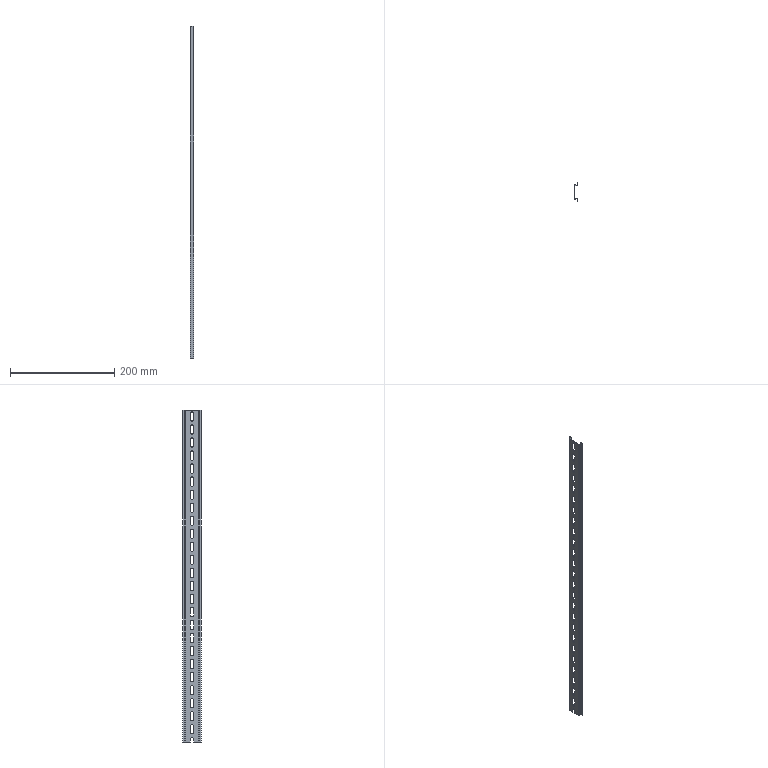Part | SolidWorks | features BaseBody 1 | 1 solid | 126 faces | box 7.5 x 35 x 637 mm | volume 27495 mm3 | plane 67 | cylinder 59 | commonest cylinder face diameters 6.3 x51 1 x4 2 x4